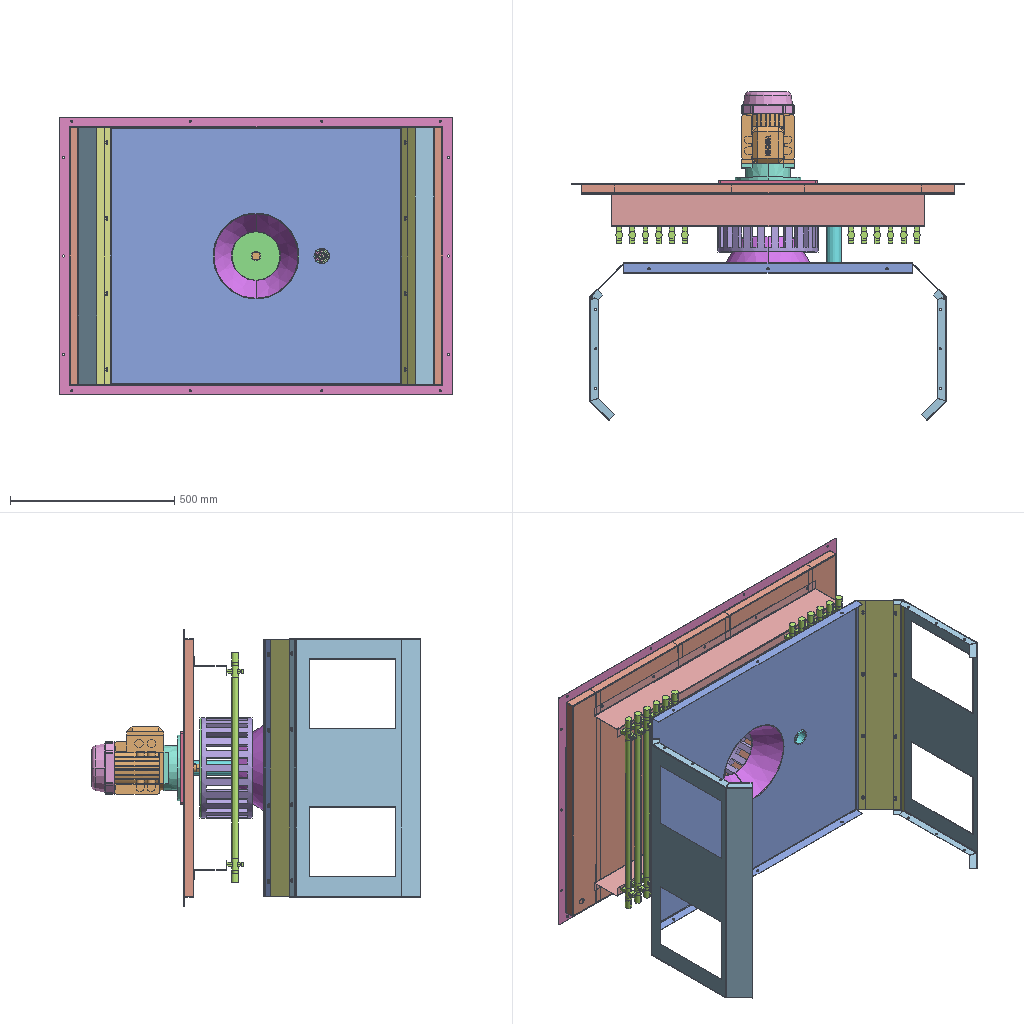Assembly | SolidWorks | 17 different items | 34 placed | box 1195 x 1000 x 845 mm
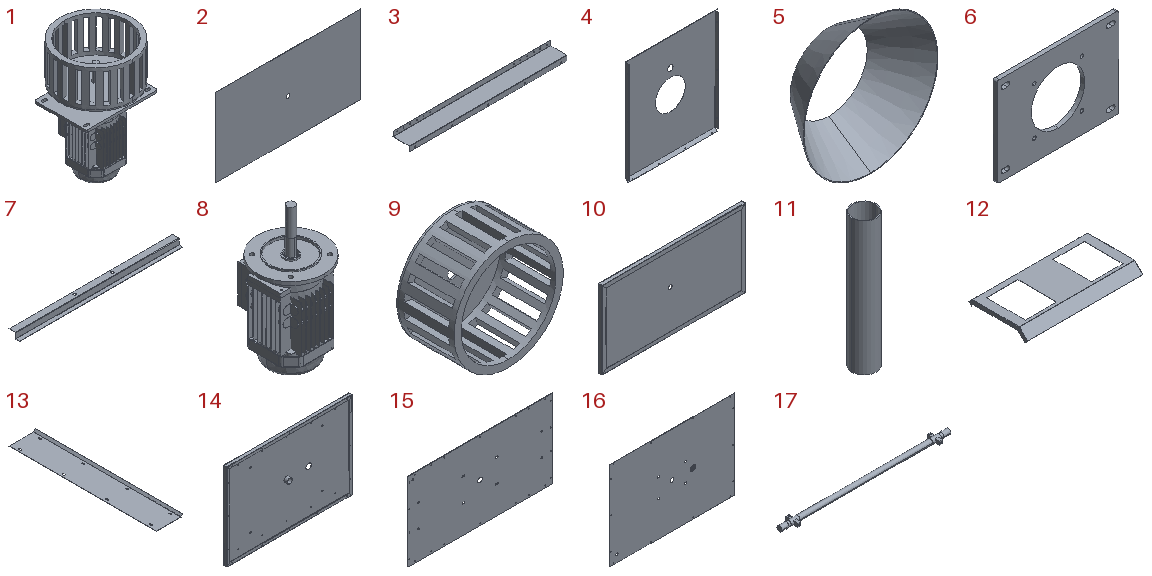Parts list (item | name | quantity | parent item | size | volume | features):
1 | (subassembly) | x1 | - | 306 x 306 x 488 mm | 7800062 mm3 | features AEMSimFeature 1
2 | - | x1 | - | 1135 x 1.2 x 615 mm | 836782 mm3 | features EdgeFlange 2, FlatPattern 1, ICE 1, SMBaseFlange 1, SheetMetal 1
3 | - | x2 | - | 950 x 100 x 58.8 mm | 177585 mm3 | features EdgeFlange 2, HoleWzd 2, FlatPattern 1, LPattern 1, SMBaseFlange 1, SheetMetal 1
4 | - | x1 | - | 780 x 30 x 921.426 mm | 870668 mm3 | features HoleWzd 3, EdgeFlange 2, Cut 1, FlatPattern 1, ICE 1, SMBaseFlange 1, SheetMetal 1
5 | - | x1 | - | 260 x 80 x 260 mm | 74495 mm3 | features Revolution 1, Shell 1
6 | - | x1 | in 1 | 300 x 10 x 220 mm | 512466 mm3 | features ICE 2, Extrusion 1, Fillet 1, HoleWzd 1
7 | - | x4 | - | 780 x 50.8 x 28 mm | 71077 mm3 | features EdgeFlange 2, FlatPattern 1, HoleWzd 1, ICE 1, SMBaseFlange 1, SheetMetal 1
8 | - | x1 | in 1 | 200 x 225.2 x 400 mm | 5238989 mm3 | features ICE 39, Fillet 15, MirrorPattern 11, Extrusion 5, Revolution 5, CirPattern 4, LibraryFeature 3, Chamfer 2, Dome 2, LPattern 2, CombineBodies 1, Shell 1
9 | - | x1 | in 1 | 306 x 160 x 306 mm | 2048607 mm3 | features ICE 3, CirPattern 1, Extrusion 1
10 | - | x1 | - | 1135 x 30 x 615 mm | 1067895 mm3 | features EdgeFlange 2, FlatPattern 1, ICE 1, SMBaseFlange 1, SheetMetal 1
11 | - | x1 | - | 45 x 45 x 245 mm | 40455 mm3 | features Extrusion 1
12 | - | x2 | - | 785 x 397.782 x 74.246 mm | 291656 mm3 | features EdgeFlange 3, HoleWzd 2, FlatPattern 1, ICE 1, SMBaseFlange 1, SheetMetal 1
13 | - | x2 | - | 140.607 x 780 x 11.455 mm | 134418 mm3 | features ICE 2, EdgeFlange 1, FlatPattern 1, LPattern 1, SMBaseFlange 1, SheetMetal 1
14 | - | x1 | - | 1135 x 31.2 x 785 mm | 1303037 mm3 | features ICE 4, EdgeFlange 2, HoleWzd 2, Cut 1, FlatPattern 1, SMBaseFlange 1, SheetMetal 1, WeldmentFeature 1
15 | - | x1 | - | 1135 x 1.2 x 615 mm | 833766 mm3 | features ICE 4, EdgeFlange 2, Fillet 1, FlatPattern 1, HoleWzd 1, SMBaseFlange 1, SheetMetal 1, WeldmentFeature 1
16 | - | x1 | - | 1195 x 1.2 x 845 mm | 1207133 mm3 | features ICE 5, EdgeFlange 2, HoleWzd 2, Fillet 1, FlatPattern 1, SMBaseFlange 1, SheetMetal 1, WeldmentFeature 1
17 | - | x12 | - | 700 x 50.5 x 21 mm | 231919 mm3 | features HoleWzd 2, ICE 2, LPattern 1, Revolution 1
Mates (type | each side: item.copy, entity, surface, feature):
In the top assembly
Width | 10.1 face | 10.1 face | 2.1 face | 2 times
Coincident | 10.1 face | 2.1 face
Parallel | 10.1 face | 2.1 face
Coincident | 2.1 face | 3.1 face plane Edge-Flange2
Coincident | 2.1 face | 3.2 face plane Edge-Flange2
Coincident | 3.1 face plane Edge-Flange1 | 3.2 face plane Edge-Flange1
Width | 3.2 face plane Base-Flange1 | 3.1 face plane Base-Flange1 | 10.1 face | 10.1 face
Coincident | 3.1 face plane Edge-Flange1 | 17.1 face plane LPattern1
Concentric | 3.1 face cylinder LPattern1 | 17.1 face cylinder M5 Clearance Hole1
Width | 3.2 face plane Edge-Flange2 | 3.2 face plane Edge-Flange2 | 2.1 face
Coincident | 3.1 face plane Edge-Flange1 | 17.2 face plane LPattern1
Concentric | 3.1 face cylinder LPattern1 | 17.2 face cylinder M5 Clearance Hole1
Parallel | 17.1 face plane LPattern1 | 17.2 face plane LPattern1
Parallel | 10.1 face | 17.1 face plane LPattern1
DistanceDim | 8.1 face plane Revolve6 | 10.1 face
Concentric | 10.1 face | 8.1 face cylinder Revolve1
Coincident | 2.1 face | 5.1 face
Coincident | 10.1 face | 5.1 face
Coincident | 2.1 face | 5.2 face
Coincident | 10.1 face | 5.2 face | 2 times
Coincident | 5.1 face | 5.2 face
DistanceDim | 4.1 face plane Base-Flange1 | 2.1 face
Concentric | 4.1 face cylinder Cut-Extrude1 | 9.1 face cylinder Boss-Extrude1
DistanceDim | 12.1 face plane Base-Flange1 | 10.1 face
Coincident | 12.1 face plane Edge-Flange1 | 13.1 face plane Base-Flange1
Coincident | 12.2 face plane Edge-Flange1 | 13.2 face plane Base-Flange1
Coincident | 4.1 face plane Base-Flange1 | 5.3 face plane Revolve1
Concentric | 4.1 face cylinder Cut-Extrude1 | 5.3 face cone Revolve1
Coincident | 2.1 face | 14.1 face plane Base-Flange1
Concentric | 8.1 edge | 14.1 edge
Coincident | 14.1 face plane Base-Flange1 | 7.1 face plane Base-Flange1
Coincident | 14.1 face plane Edge-Flange1 | 7.1 face plane Base-Flange1
Coincident | 7.1 face plane Base-Flange1 | 7.2 face plane Base-Flange1
DistanceDim | 7.2 face plane Edge-Flange1 | 14.1 face plane Edge-Flange1 | 2 times
DistanceDim | 7.1 face plane Edge-Flange1 | 14.1 face plane Edge-Flange1
Coincident | 14.1 face plane Edge-Flange2 | 15.1 face plane Base-Flange1
Coincident | 14.1 face plane Edge-Flange1 | 15.1 face plane Base-Flange1 | 2 times
Concentric | 8.1 face cylinder Revolve6 | 16.1 face cylinder Cut-Extrude1
Parallel | 14.1 face plane Edge-Flange1 | 16.1 face plane Base-Flange1
Slot | 13.1 face cylinder Cut-Extrude3 | 4.1 face cylinder M5 Clearance Hole2
Slot | 13.1 face cylinder LPattern1 | 4.1 face cylinder M5 Clearance Hole2
Slot | 13.2 face cylinder Cut-Extrude3 | 4.1 face cylinder M5 Clearance Hole1
Slot | 13.2 face cylinder LPattern1 | 4.1 face cylinder M5 Clearance Hole1
Slot | 12.2 face cylinder M5 Clearance Hole2 | 13.2 face cylinder LPattern1
Parallel | 4.1 face plane Edge-Flange2 | 16.1 face plane Base-Flange1
Coincident | 14.1 face plane Edge-Flange2 | 16.1 face plane Base-Flange1
Concentric | 14.1 face cylinder Cut-Extrude4 | 11.1 face cylinder Boss-Extrude1
Coincident | 16.1 face plane Base-Flange1 | 11.1 face plane Boss-Extrude1
Coincident | 3.2 face plane Edge-Flange1 | 17.1 face plane Boss-Extrude1
Concentric | 3.2 face cylinder M6 Clearance Hole1 | 14.1 edge
Coincident | 3.2 face plane Edge-Flange2 | 14.1 face plane Base-Flange1
Concentric | 3.2 face cylinder M6 Clearance Hole1 | 14.1 face cylinder M5 Clearance Hole1
Coincident | 6.1 face plane Boss-Extrude1 | 16.1 face plane Base-Flange1
Concentric | 3.1 face cylinder M6 Clearance Hole1 | 14.1 face cylinder M5 Clearance Hole1
Coincident | 4.1 face plane Edge-Flange3 | 13.1 face plane Base-Flange1
Slot | 13.1 face cylinder LPattern1 | 12.1 face cylinder M5 Clearance Hole2
Slot | 12.1 face cylinder M5 Clearance Hole2 | 13.1 face cylinder Cut-Extrude3
Coincident | 4.1 face plane Edge-Flange3 | 13.2 face plane Base-Flange1
DistanceDim | 4.1 face plane Base-Flange1 | 14.1 face plane Base-Flange1
Parallel | 12.2 face plane Base-Flange1 | 12.1 face plane Base-Flange1
Parallel | 12.2 face plane Base-Flange1 | 14.1 face plane Edge-Flange1
In subassembly 1
DistanceDim | 9.2 face plane Boss-Extrude2 | 8.2 face plane Revolve6
Concentric | 8.2 face cylinder Revolve1 | 9.2 face cylinder Cut-Extrude2
Coincident | 8.2 face plane Revolve6 | 6.2 face plane Boss-Extrude1
Concentric | 8.2 face cylinder Revolve1 | 6.2 face cylinder Cut-Extrude1
Parallel | 8.2 face plane Boss-Extrude27 | 6.2 face plane Boss-Extrude1